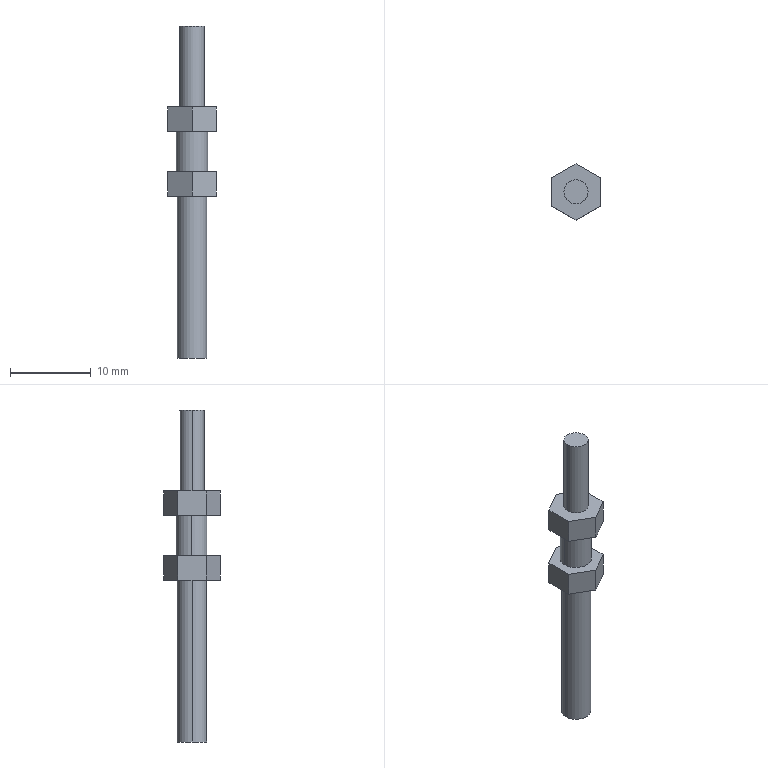Part | STEP file | ASND-0110-7.1aq | 3 solids | 26 faces | box 6 x 6.928 x 41 mm | volume 521.465 mm3 | plane 20 | cylinder 6 | commonest cylinder face diameters 3 x2 3.615 x2 3.859 x2